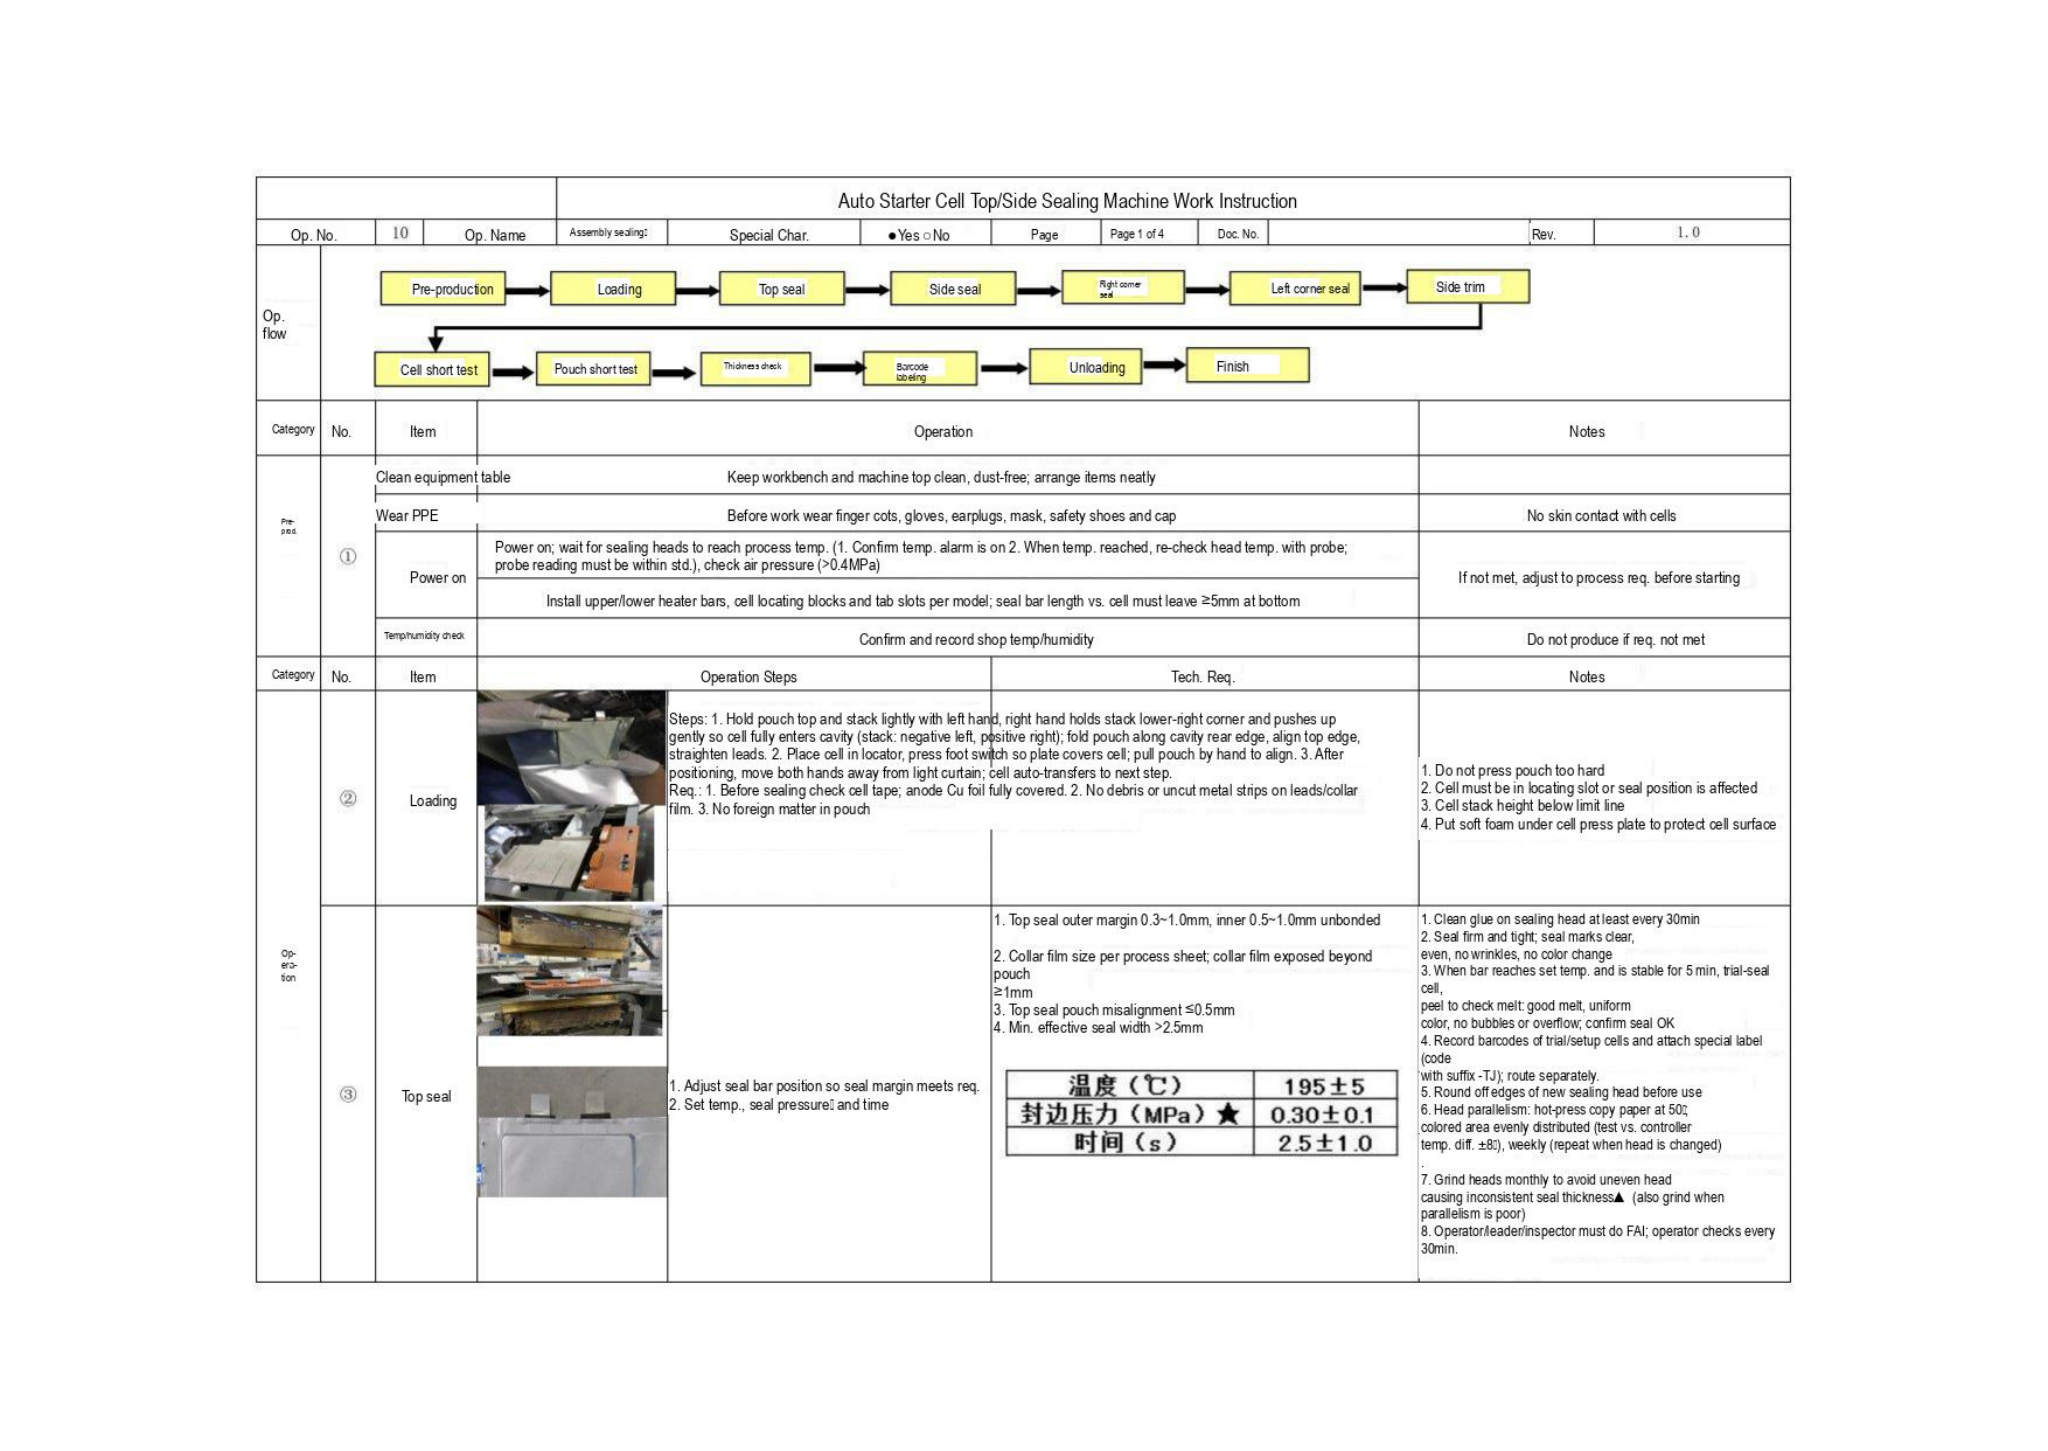Auto Starter Cell Top/Side Sealing Machine Work Instruction

| Op. No. | 10 | Op. Name | Assembly sealing | Special Char. | ●Yes ○No | Page | Page 1 of 4 | Doc. No. | | Rev. | 1.0 |
|---|---|---|---|---|---|---|---|---|---|---|---|

Op. flow

Pre-production → Loading → Top seal → Side seal → Right corner seal → Left corner seal → Side trim → Cell short test → Pouch short test → Thickness check → Barcode labeling → Unloading → Finish

| Category | No. | Item | Operation | Notes |
|---|---|---|---|---|
| Pre-prod. | ① | Clean equipment table | Keep workbench and machine top clean, dust-free; arrange items neatly | |
| | | Wear PPE | Before work wear finger cots, gloves, earplugs, mask, safety shoes and cap | No skin contact with cells |
| | | Power on | Power on; wait for sealing heads to reach process temp. (1. Confirm temp. alarm is on 2. When temp. reached, re-check head temp. with probe; probe reading must be within std.), check air pressure (>0.4MPa) | If not met, adjust to process req. before starting |
| | | | Install upper/lower heater bars, cell locating blocks and tab slots per model; seal bar length vs. cell must leave ≥5mm at bottom | |
| | | Temp/humidity check | Confirm and record shop temp/humidity | Do not produce if req. not met |

| Category | No. | Item | Operation Steps | Tech. Req. | Notes |
|---|---|---|---|---|---|
| Operation | ② | Loading | Steps: 1. Hold pouch top and stack lightly with left hand, right hand holds stack lower-right corner and pushes up gently so cell fully enters cavity (stack: negative left, positive right); fold pouch along cavity rear edge, align top edge, straighten leads. 2. Place cell in locator, press foot switch so plate covers cell; pull pouch by hand to align. 3. After positioning, move both hands away from light curtain; cell auto-transfers to next step.<br>Req.: 1. Before sealing check cell tape; anode Cu foil fully covered. 2. No debris or uncut metal strips on leads/collar film. 3. No foreign matter in pouch | | 1. Do not press pouch too hard<br>2. Cell must be in locating slot or seal position is affected<br>3. Cell stack height below limit line<br>4. Put soft foam under cell press plate to protect cell surface |
| | ③ | Top seal | 1. Adjust seal bar position so seal margin meets req.<br>2. Set temp., seal pressure and time | 1. Top seal outer margin 0.3~1.0mm, inner 0.5~1.0mm unbonded<br>2. Collar film size per process sheet; collar film exposed beyond pouch ≥1mm<br>3. Top seal pouch misalignment ≤0.5mm<br>4. Min. effective seal width >2.5mm<br><br>温度（℃） 195±5<br>封边压力（MPa）★ 0.30±0.1<br>时间（s） 2.5±1.0 | 1. Clean glue on sealing head at least every 30min<br>2. Seal firm and tight; seal marks clear, even, no wrinkles, no color change<br>3. When bar reaches set temp. and is stable for 5 min, trial-seal cell, peel to check melt: good melt, uniform color, no bubbles or overflow; confirm seal OK<br>4. Record barcodes of trial/setup cells and attach special label (code with suffix -TJ); route separately.<br>5. Round off edges of new sealing head before use<br>6. Head parallelism: hot-press copy paper at 50; colored area evenly distributed (test vs. controller temp. diff. ±8), weekly (repeat when head is changed)<br>7. Grind heads monthly to avoid uneven head causing inconsistent seal thickness▲ (also grind when parallelism is poor)<br>8. Operator/leader/inspector must do FAI; operator checks every 30min. |
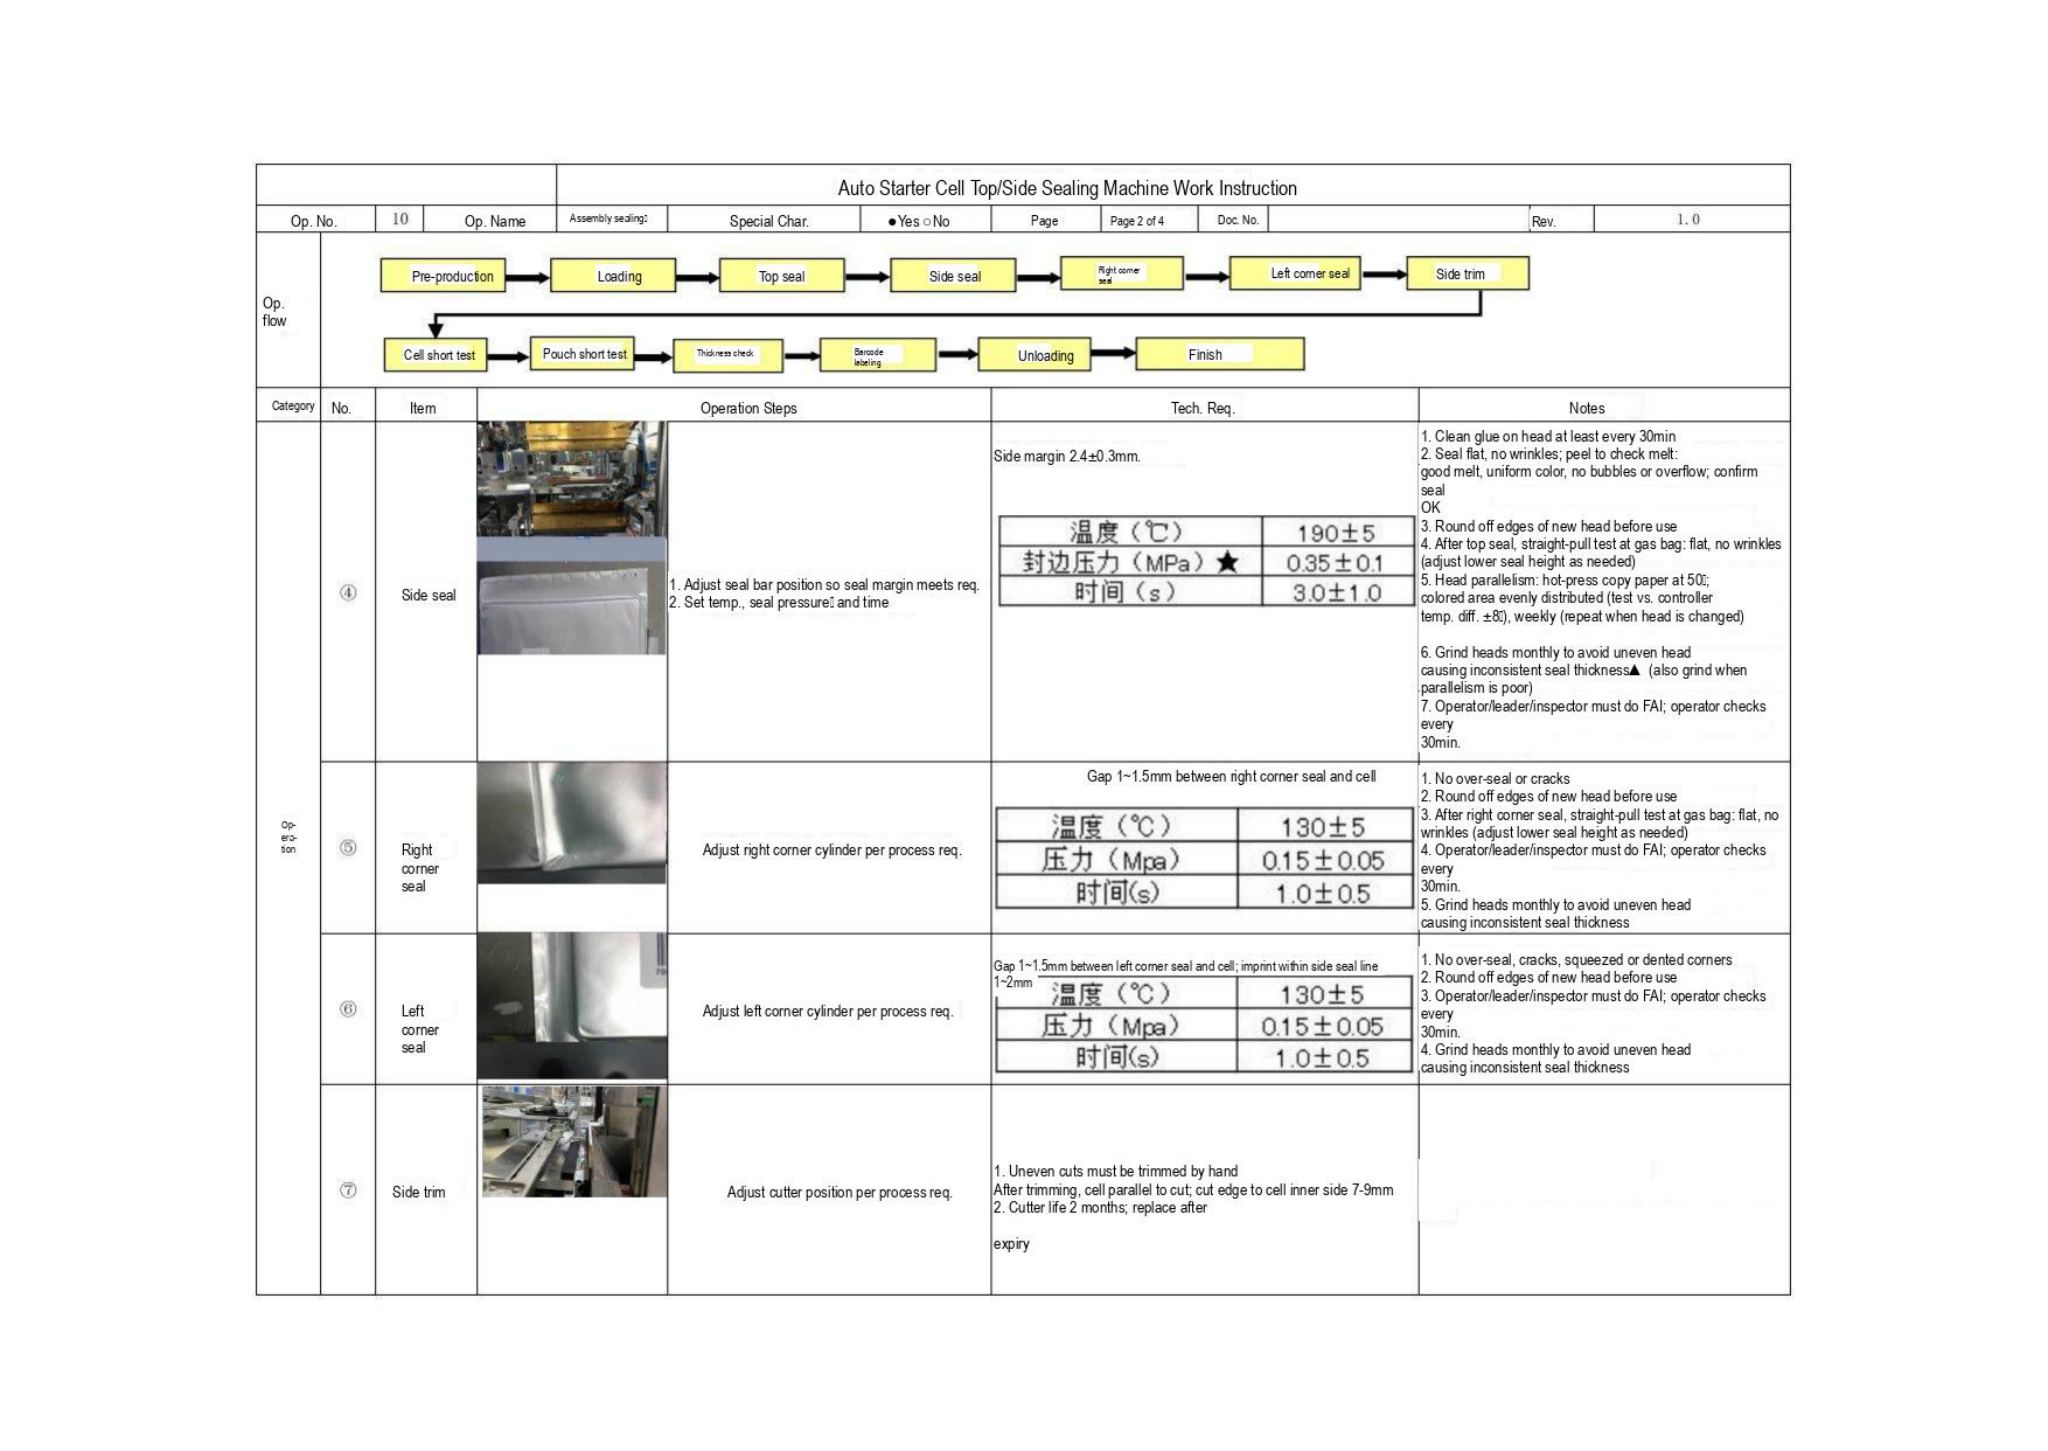Auto Starter Cell Top/Side Sealing Machine Work Instruction

| Op. No. | 10 | Op. Name | Assembly sealing | Special Char. | ●Yes ○No | Page | Page 2 of 4 | Doc. No. | | Rev. | 1.0 |
|---|---|---|---|---|---|---|---|---|---|---|---|

Op. flow

Pre-production → Loading → Top seal → Side seal → Right corner seal → Left corner seal → Side trim → Cell short test → Pouch short test → Thickness check → Barcode labeling → Unloading → Finish

| Category | No. | Item | Operation Steps | Tech. Req. | Notes |
|---|---|---|---|---|---|
| Op-era-tion | ④ | Side seal | 1. Adjust seal bar position so seal margin meets req.<br>2. Set temp., seal pressure and time | Side margin 2.4±0.3mm.<br><br>温度（℃） 190±5<br>封边压力（MPa）★ 0.35±0.1<br>时间（s） 3.0±1.0 | 1. Clean glue on head at least every 30min<br>2. Seal flat, no wrinkles; peel to check melt: good melt, uniform color, no bubbles or overflow; confirm seal OK<br>3. Round off edges of new head before use<br>4. After top seal, straight-pull test at gas bag: flat, no wrinkles (adjust lower seal height as needed)<br>5. Head parallelism: hot-press copy paper at 50; colored area evenly distributed (test vs. controller temp. diff. ±8), weekly (repeat when head is changed)<br>6. Grind heads monthly to avoid uneven head causing inconsistent seal thickness▲ (also grind when parallelism is poor)<br>7. Operator/leader/inspector must do FAI; operator checks every 30min. |
| | ⑤ | Right corner seal | Adjust right corner cylinder per process req. | Gap 1~1.5mm between right corner seal and cell<br><br>温度（℃） 130±5<br>压力（Mpa） 0.15±0.05<br>时间(s) 1.0±0.5 | 1. No over-seal or cracks<br>2. Round off edges of new head before use<br>3. After right corner seal, straight-pull test at gas bag: flat, no wrinkles (adjust lower seal height as needed)<br>4. Operator/leader/inspector must do FAI; operator checks every 30min.<br>5. Grind heads monthly to avoid uneven head causing inconsistent seal thickness |
| | ⑥ | Left corner seal | Adjust left corner cylinder per process req. | Gap 1~1.5mm between left corner seal and cell; imprint within side seal line 1~2mm<br>温度（℃） 130±5<br>压力（Mpa） 0.15±0.05<br>时间(s) 1.0±0.5 | 1. No over-seal, cracks, squeezed or dented corners<br>2. Round off edges of new head before use<br>3. Operator/leader/inspector must do FAI; operator checks every 30min.<br>4. Grind heads monthly to avoid uneven head causing inconsistent seal thickness |
| | ⑦ | Side trim | Adjust cutter position per process req. | 1. Uneven cuts must be trimmed by hand<br>After trimming, cell parallel to cut; cut edge to cell inner side 7-9mm<br>2. Cutter life 2 months; replace after<br><br>expiry | |
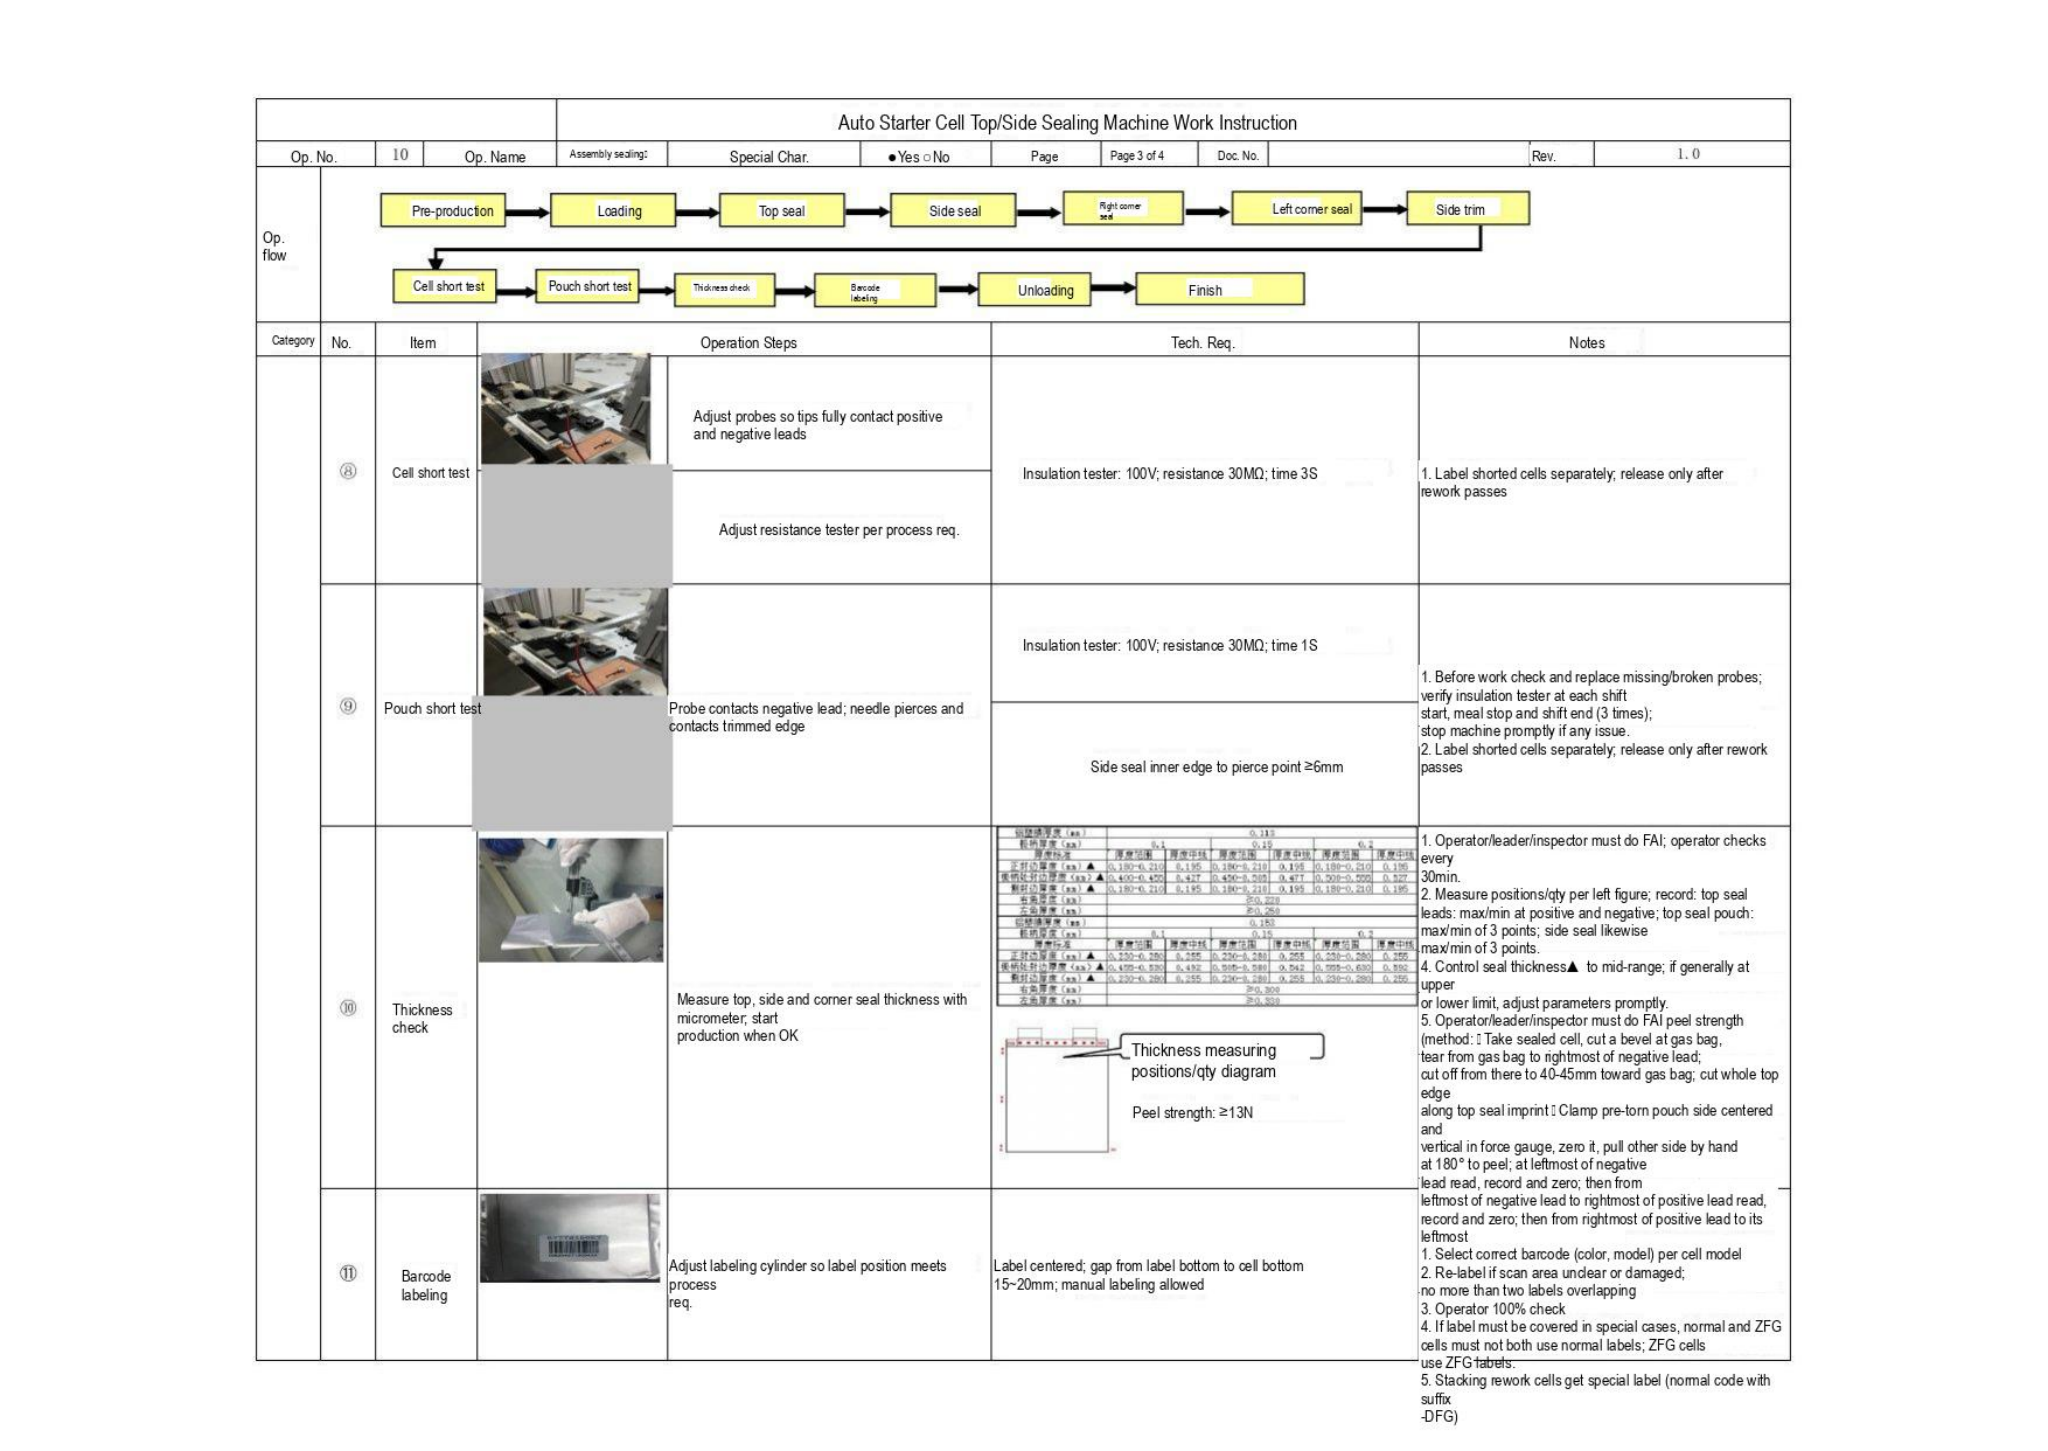Auto Starter Cell Top/Side Sealing Machine Work Instruction

| Op. No. | 10 | Op. Name | Assembly sealing: | Special Char. | ●Yes ○No | Page | Page 3 of 4 | Doc. No. | | Rev. | 1.0 |
|---|---|---|---|---|---|---|---|---|---|---|---|

Op. flow

Pre-production → Loading → Top seal → Side seal → Right corner seal → Left corner seal → Side trim → Cell short test → Pouch short test → Thickness check → Barcode labeling → Unloading → Finish

| Category | No. | Item | Operation Steps | Tech. Req. | Notes |
|---|---|---|---|---|---|
| | ⑧ | Cell short test | Adjust probes so tips fully contact positive and negative leads<br><br>Adjust resistance tester per process req. | Insulation tester: 100V; resistance 30MΩ; time 3S | 1. Label shorted cells separately; release only after rework passes |
| | ⑨ | Pouch short test | Probe contacts negative lead; needle pierces and contacts trimmed edge | Insulation tester: 100V; resistance 30MΩ; time 1S<br><br>Side seal inner edge to pierce point ≥6mm | 1. Before work check and replace missing/broken probes; verify insulation tester at each shift start, meal stop and shift end (3 times); stop machine promptly if any issue.<br>2. Label shorted cells separately; release only after rework passes |
| | ⑩ | Thickness check | Measure top, side and corner seal thickness with micrometer; start production when OK | (see table below)<br><br>Thickness measuring positions/qty diagram<br><br>Peel strength: ≥13N | 1. Operator/leader/inspector must do FAI; operator checks every 30min.<br>2. Measure positions/qty per left figure; record: top seal leads: max/min at positive and negative; top seal pouch: max/min of 3 points; side seal likewise max/min of 3 points.<br>4. Control seal thickness▲ to mid-range; if generally at upper or lower limit, adjust parameters promptly.<br>5. Operator/leader/inspector must do FAI peel strength (method: Take sealed cell, cut a bevel at gas bag, tear from gas bag to rightmost of negative lead; cut off from there to 40-45mm toward gas bag; cut whole top edge along top seal imprint Clamp pre-torn pouch side centered and vertical in force gauge, zero it, pull other side by hand at 180° to peel; at leftmost of negative lead read, record and zero; then from leftmost of negative lead to rightmost of positive lead read, record and zero; then from rightmost of positive lead to its leftmost |
| | ⑪ | Barcode labeling | Adjust labeling cylinder so label position meets process req. | Label centered; gap from label bottom to cell bottom 15~20mm; manual labeling allowed | 1. Select correct barcode (color, model) per cell model<br>2. Re-label if scan area unclear or damaged; no more than two labels overlapping<br>3. Operator 100% check<br>4. If label must be covered in special cases, normal and ZFG cells must not both use normal labels; ZFG cells use ZFG labels.<br>5. Stacking rework cells get special label (normal code with suffix -DFG) |

| 铝塑膜厚度(mm) | 0.113 | | | | | |
|---|---|---|---|---|---|---|
| 极耳厚度(mm) | 0.1 | | 0.15 | | 0.2 | |
| 厚度标准 | 厚度范围 | 厚度中线 | 厚度范围 | 厚度中线 | 厚度范围 | 厚度中线 |
| 正封边厚度(mm)▲ | 0.180~0.210 | 0.195 | 0.180~0.210 | 0.195 | 0.180~0.210 | 0.195 |
| 极耳处封边厚度(mm)▲ | 0.400~0.450 | 0.427 | 0.450~0.505 | 0.477 | 0.500~0.555 | 0.527 |
| 侧封边厚度(mm)▲ | 0.180~0.210 | 0.195 | 0.180~0.210 | 0.195 | 0.180~0.210 | 0.195 |
| 右角厚度(mm) | ≥0.220 | | | | | |
| 左角厚度(mm) | ≥0.250 | | | | | |
| 铝塑膜厚度(mm) | 0.153 | | | | | |
| 极耳厚度(mm) | 0.1 | | 0.15 | | 0.2 | |
| 厚度标准 | 厚度范围 | 厚度中线 | 厚度范围 | 厚度中线 | 厚度范围 | 厚度中线 |
| 正封边厚度(mm)▲ | 0.230~0.280 | 0.255 | 0.230~0.280 | 0.255 | 0.230~0.280 | 0.255 |
| 极耳处封边厚度(mm)▲ | 0.455~0.530 | 0.492 | 0.505~0.580 | 0.542 | 0.555~0.630 | 0.592 |
| 侧封边厚度(mm)▲ | 0.230~0.280 | 0.255 | 0.230~0.280 | 0.255 | 0.230~0.280 | 0.255 |
| 右角厚度(mm) | ≥0.300 | | | | | |
| 左角厚度(mm) | ≥0.330 | | | | | |
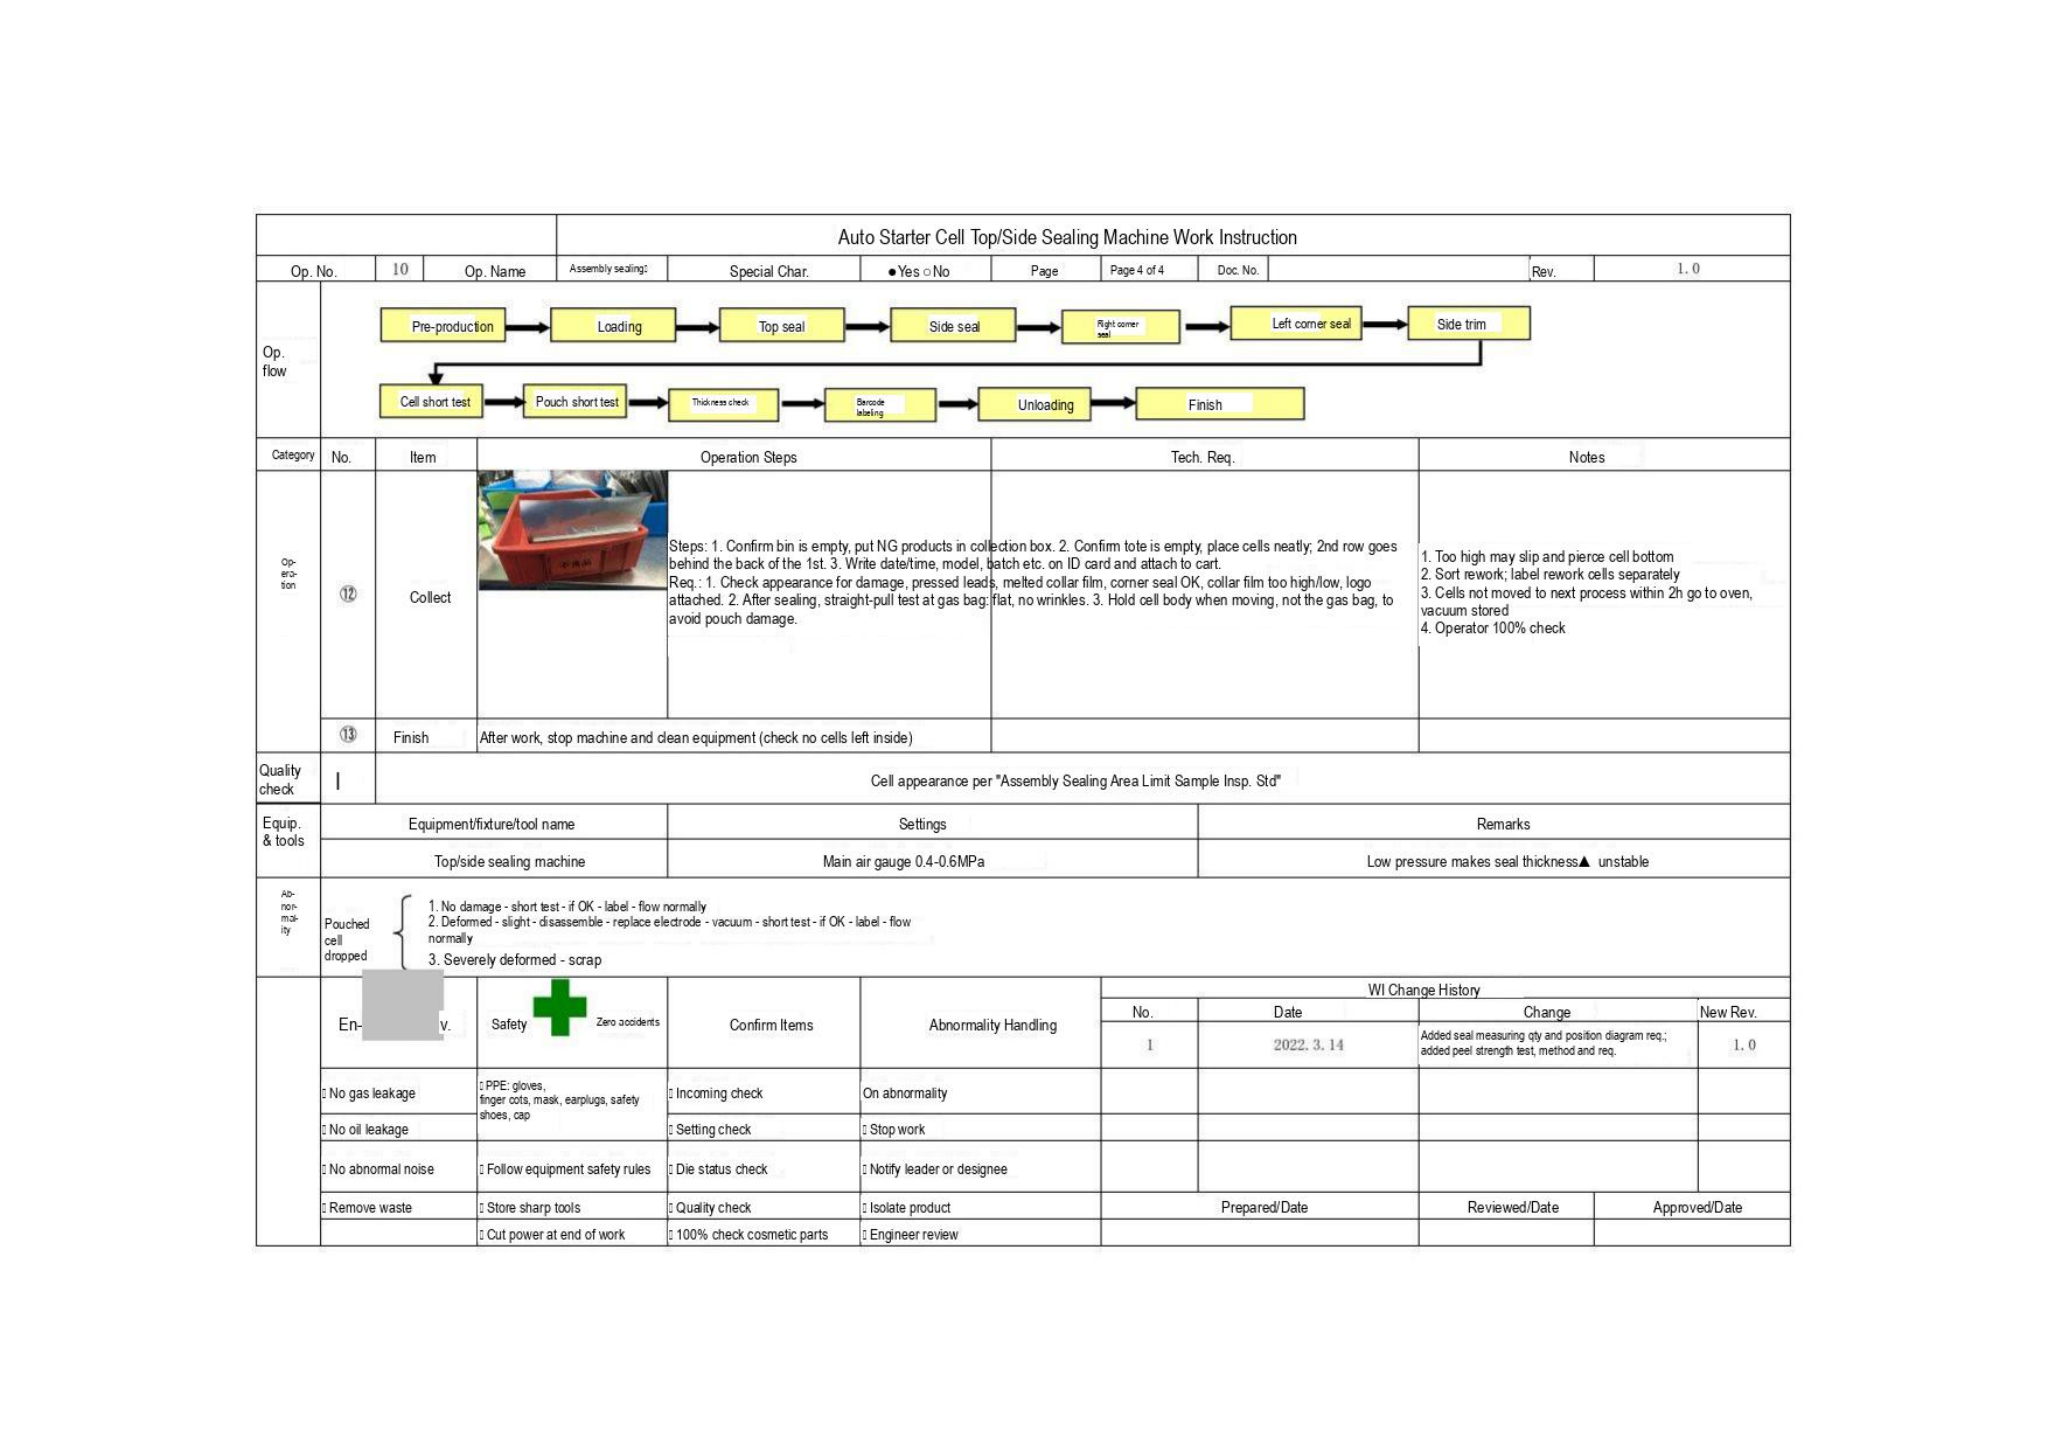# Auto Starter Cell Top/Side Sealing Machine Work Instruction

| Op. No. | 10 | Op. Name | Assembly sealing: | Special Char. | ●Yes ○No | Page | Page 4 of 4 | Doc. No. | | Rev. | 1.0 |
|---|---|---|---|---|---|---|---|---|---|---|---|

**Op. flow**

Pre-production → Loading → Top seal → Side seal → Right corner seal → Left corner seal → Side trim → Cell short test → Pouch short test → Thickness check → Barcode labeling → Unloading → Finish

| Category | No. | Item | Operation Steps | Tech. Req. | Notes |
|---|---|---|---|---|---|
| Op-era-tion | ⑫ | Collect | Steps: 1. Confirm bin is empty, put NG products in collection box. 2. Confirm tote is empty, place cells neatly; 2nd row goes behind the back of the 1st. 3. Write date/time, model, batch etc. on ID card and attach to cart.<br>Req.: 1. Check appearance for damage, pressed leads, melted collar film, corner seal OK, collar film too high/low, logo attached. 2. After sealing, straight-pull test at gas bag: flat, no wrinkles. 3. Hold cell body when moving, not the gas bag, to avoid pouch damage. | | 1. Too high may slip and pierce cell bottom<br>2. Sort rework; label rework cells separately<br>3. Cells not moved to next process within 2h go to oven, vacuum stored<br>4. Operator 100% check |
| | ⑬ | Finish | After work, stop machine and clean equipment (check no cells left inside) | | |
| Quality check | I | Cell appearance per "Assembly Sealing Area Limit Sample Insp. Std" | | | |

| Equip. & tools | Equipment/fixture/tool name | Settings | Remarks |
|---|---|---|---|
| | Top/side sealing machine | Main air gauge 0.4-0.6MPa | Low pressure makes seal thickness▲ unstable |

**Ab-nor-mal-ity**

Pouched cell dropped
1. No damage - short test - if OK - label - flow normally
2. Deformed - slight - disassemble - replace electrode - vacuum - short test - if OK - label - flow normally
3. Severely deformed - scrap

| En- v. | Safety Zero accidents | Confirm Items | Abnormality Handling |
|---|---|---|---|
| □ No gas leakage | □ PPE: gloves, finger cots, mask, earplugs, safety shoes, cap | □ Incoming check | On abnormality |
| □ No oil leakage | | □ Setting check | □ Stop work |
| □ No abnormal noise | □ Follow equipment safety rules | □ Die status check | □ Notify leader or designee |
| □ Remove waste | □ Store sharp tools | □ Quality check | □ Isolate product |
| | □ Cut power at end of work | □ 100% check cosmetic parts | □ Engineer review |

**WI Change History**

| No. | Date | Change | New Rev. |
|---|---|---|---|
| 1 | 2022. 3. 14 | Added seal measuring qty and position diagram req.; added peel strength test, method and req. | 1.0 |
| | | | |
| | | | |
| | | | |

| Prepared/Date | Reviewed/Date | Approved/Date |
|---|---|---|
| | | |